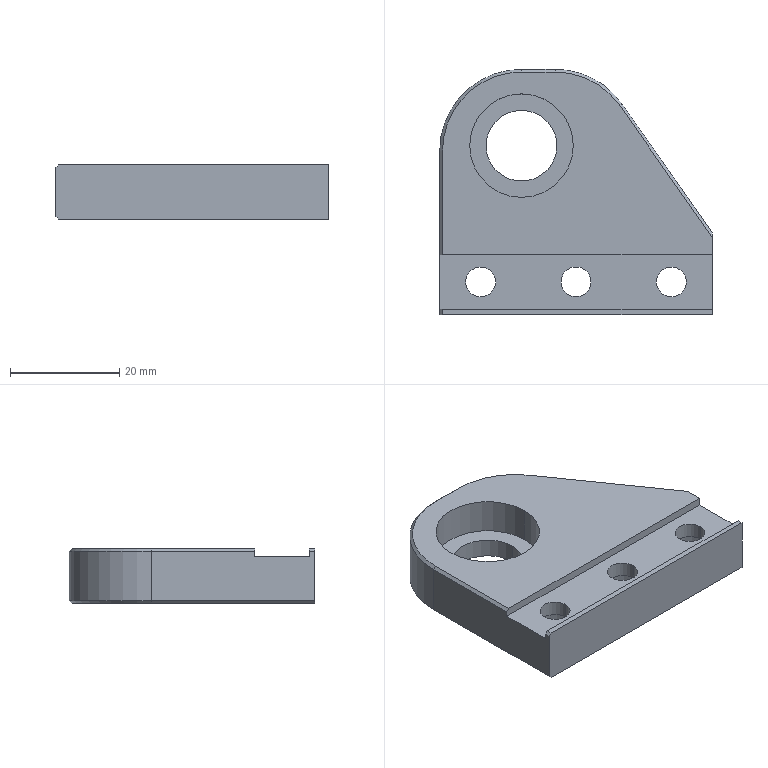Part | STEP file | 10000020492swp000-1 | 1 solid | 44 faces | box 50 x 45 x 10 mm | volume 14150 mm3 | plane 22 | cylinder 18 | cone 4 | commonest cylinder face diameters 5.5 x6 10 x6 13 x2 19 x2 30 x2
STEP:
#1=CARTESIAN_POINT('',(-19.5,8.5,3.5));
#2=VERTEX_POINT('',#1);
#3=CARTESIAN_POINT('',(-0.5,8.5,3.5));
#4=VERTEX_POINT('',#3);
#5=CARTESIAN_POINT('',(-10.,8.5,3.5));
#6=DIRECTION('',(0.,0.,1.));
#7=DIRECTION('',(1.,0.,0.));
#8=AXIS2_PLACEMENT_3D('',#5,#6,#7);
#9=CIRCLE('',#8,9.5);
#10=EDGE_CURVE('',#2,#4,#9,.T.);
#11=ORIENTED_EDGE('',*,*,#10,.F.);
#12=CARTESIAN_POINT('',(-19.5,8.5,10.));
#13=VERTEX_POINT('',#12);
#14=CARTESIAN_POINT('',(-19.5,8.5,10.));
#15=DIRECTION('',(0.,0.,1.));
#16=VECTOR('',#15,1000.);
#17=LINE('',#14,#16);
#18=EDGE_CURVE('',#2,#13,#17,.T.);
#19=ORIENTED_EDGE('',*,*,#18,.T.);
#20=CARTESIAN_POINT('',(-0.5,8.5,10.));
#21=VERTEX_POINT('',#20);
#22=CARTESIAN_POINT('',(-10.,8.5,10.));
#23=DIRECTION('',(0.,0.,1.));
#24=DIRECTION('',(1.,0.,0.));
#25=AXIS2_PLACEMENT_3D('',#22,#23,#24);
#26=CIRCLE('',#25,9.5);
#27=EDGE_CURVE('',#13,#21,#26,.T.);
#28=ORIENTED_EDGE('',*,*,#27,.T.);
#29=CARTESIAN_POINT('',(-0.5,8.5,10.));
#30=DIRECTION('',(0.,0.,1.));
#31=VECTOR('',#30,1000.);
#32=LINE('',#29,#31);
#33=EDGE_CURVE('',#4,#21,#32,.T.);
#34=ORIENTED_EDGE('',*,*,#33,.F.);
#35=EDGE_LOOP('',(#11,#19,#28,#34));
#36=FACE_OUTER_BOUND('',#35,.T.);
#37=CARTESIAN_POINT('',(-10.,8.5,10.));
#38=DIRECTION('',(0.,0.,1.));
#39=DIRECTION('',(1.,0.,0.));
#40=AXIS2_PLACEMENT_3D('',#37,#38,#39);
#41=CYLINDRICAL_SURFACE('',#40,9.5);
#42=ADVANCED_FACE('',(#36),#41,.F.);
#43=CARTESIAN_POINT('',(-16.5,8.5,0.));
#44=VERTEX_POINT('',#43);
#45=CARTESIAN_POINT('',(-3.5,8.5,0.));
#46=VERTEX_POINT('',#45);
#47=CARTESIAN_POINT('',(-10.,8.5,0.));
#48=DIRECTION('',(0.,0.,1.));
#49=DIRECTION('',(1.,0.,0.));
#50=AXIS2_PLACEMENT_3D('',#47,#48,#49);
#51=CIRCLE('',#50,6.5);
#52=EDGE_CURVE('',#44,#46,#51,.T.);
#53=ORIENTED_EDGE('',*,*,#52,.F.);
#54=CARTESIAN_POINT('',(-16.5,8.5,3.5));
#55=VERTEX_POINT('',#54);
#56=CARTESIAN_POINT('',(-16.5,8.5,10.));
#57=DIRECTION('',(0.,0.,1.));
#58=VECTOR('',#57,1000.);
#59=LINE('',#56,#58);
#60=EDGE_CURVE('',#44,#55,#59,.T.);
#61=ORIENTED_EDGE('',*,*,#60,.T.);
#62=CARTESIAN_POINT('',(-3.5,8.5,3.5));
#63=VERTEX_POINT('',#62);
#64=CARTESIAN_POINT('',(-10.,8.5,3.5));
#65=DIRECTION('',(0.,0.,1.));
#66=DIRECTION('',(1.,0.,0.));
#67=AXIS2_PLACEMENT_3D('',#64,#65,#66);
#68=CIRCLE('',#67,6.5);
#69=EDGE_CURVE('',#55,#63,#68,.T.);
#70=ORIENTED_EDGE('',*,*,#69,.T.);
#71=CARTESIAN_POINT('',(-3.5,8.5,10.));
#72=DIRECTION('',(0.,0.,1.));
#73=VECTOR('',#72,1000.);
#74=LINE('',#71,#73);
#75=EDGE_CURVE('',#46,#63,#74,.T.);
#76=ORIENTED_EDGE('',*,*,#75,.F.);
#77=EDGE_LOOP('',(#53,#61,#70,#76));
#78=FACE_OUTER_BOUND('',#77,.T.);
#79=CARTESIAN_POINT('',(-10.,8.5,10.));
#80=DIRECTION('',(0.,0.,1.));
#81=DIRECTION('',(1.,0.,0.));
#82=AXIS2_PLACEMENT_3D('',#79,#80,#81);
#83=CYLINDRICAL_SURFACE('',#82,6.5);
#84=ADVANCED_FACE('',(#78),#83,.F.);
#85=CARTESIAN_POINT('',(-12.5,-16.5,5.7));
#86=VERTEX_POINT('',#85);
#87=CARTESIAN_POINT('',(-22.5,-16.5,5.7));
#88=VERTEX_POINT('',#87);
#89=CARTESIAN_POINT('',(-17.5,-16.5,5.7));
#90=DIRECTION('',(0.,0.,-1.));
#91=DIRECTION('',(-1.,0.,0.));
#92=AXIS2_PLACEMENT_3D('',#89,#90,#91);
#93=CIRCLE('',#92,5.);
#94=EDGE_CURVE('',#86,#88,#93,.T.);
#95=ORIENTED_EDGE('',*,*,#94,.F.);
#96=CARTESIAN_POINT('',(-12.5,-16.5,0.));
#97=VERTEX_POINT('',#96);
#98=CARTESIAN_POINT('',(-12.5,-16.5,0.));
#99=DIRECTION('',(0.,0.,-1.));
#100=VECTOR('',#99,1000.);
#101=LINE('',#98,#100);
#102=EDGE_CURVE('',#86,#97,#101,.T.);
#103=ORIENTED_EDGE('',*,*,#102,.T.);
#104=CARTESIAN_POINT('',(-22.5,-16.5,0.));
#105=VERTEX_POINT('',#104);
#106=CARTESIAN_POINT('',(-17.5,-16.5,0.));
#107=DIRECTION('',(0.,0.,-1.));
#108=DIRECTION('',(-1.,0.,0.));
#109=AXIS2_PLACEMENT_3D('',#106,#107,#108);
#110=CIRCLE('',#109,5.);
#111=EDGE_CURVE('',#97,#105,#110,.T.);
#112=ORIENTED_EDGE('',*,*,#111,.T.);
#113=CARTESIAN_POINT('',(-22.5,-16.5,0.));
#114=DIRECTION('',(0.,0.,-1.));
#115=VECTOR('',#114,1000.);
#116=LINE('',#113,#115);
#117=EDGE_CURVE('',#88,#105,#116,.T.);
#118=ORIENTED_EDGE('',*,*,#117,.F.);
#119=EDGE_LOOP('',(#95,#103,#112,#118));
#120=FACE_OUTER_BOUND('',#119,.T.);
#121=CARTESIAN_POINT('',(-17.5,-16.5,0.));
#122=DIRECTION('',(0.,0.,-1.));
#123=DIRECTION('',(-1.,0.,0.));
#124=AXIS2_PLACEMENT_3D('',#121,#122,#123);
#125=CYLINDRICAL_SURFACE('',#124,5.);
#126=ADVANCED_FACE('',(#120),#125,.F.);
#127=CARTESIAN_POINT('',(-14.75,-16.5,8.5));
#128=VERTEX_POINT('',#127);
#129=CARTESIAN_POINT('',(-20.25,-16.5,8.5));
#130=VERTEX_POINT('',#129);
#131=CARTESIAN_POINT('',(-17.5,-16.5,8.5));
#132=DIRECTION('',(0.,0.,-1.));
#133=DIRECTION('',(-1.,0.,0.));
#134=AXIS2_PLACEMENT_3D('',#131,#132,#133);
#135=CIRCLE('',#134,2.75);
#136=EDGE_CURVE('',#128,#130,#135,.T.);
#137=ORIENTED_EDGE('',*,*,#136,.F.);
#138=CARTESIAN_POINT('',(-14.75,-16.5,5.7));
#139=VERTEX_POINT('',#138);
#140=CARTESIAN_POINT('',(-14.75,-16.5,0.));
#141=DIRECTION('',(0.,0.,-1.));
#142=VECTOR('',#141,1000.);
#143=LINE('',#140,#142);
#144=EDGE_CURVE('',#128,#139,#143,.T.);
#145=ORIENTED_EDGE('',*,*,#144,.T.);
#146=CARTESIAN_POINT('',(-20.25,-16.5,5.7));
#147=VERTEX_POINT('',#146);
#148=CARTESIAN_POINT('',(-17.5,-16.5,5.7));
#149=DIRECTION('',(0.,0.,-1.));
#150=DIRECTION('',(-1.,0.,0.));
#151=AXIS2_PLACEMENT_3D('',#148,#149,#150);
#152=CIRCLE('',#151,2.75);
#153=EDGE_CURVE('',#139,#147,#152,.T.);
#154=ORIENTED_EDGE('',*,*,#153,.T.);
#155=CARTESIAN_POINT('',(-20.25,-16.5,0.));
#156=DIRECTION('',(0.,0.,-1.));
#157=VECTOR('',#156,1000.);
#158=LINE('',#155,#157);
#159=EDGE_CURVE('',#130,#147,#158,.T.);
#160=ORIENTED_EDGE('',*,*,#159,.F.);
#161=EDGE_LOOP('',(#137,#145,#154,#160));
#162=FACE_OUTER_BOUND('',#161,.T.);
#163=CARTESIAN_POINT('',(-17.5,-16.5,0.));
#164=DIRECTION('',(0.,0.,-1.));
#165=DIRECTION('',(-1.,0.,0.));
#166=AXIS2_PLACEMENT_3D('',#163,#164,#165);
#167=CYLINDRICAL_SURFACE('',#166,2.75);
#168=ADVANCED_FACE('',(#162),#167,.F.);
#169=CARTESIAN_POINT('',(5.,-16.5,5.7));
#170=VERTEX_POINT('',#169);
#171=CARTESIAN_POINT('',(-5.,-16.5,5.7));
#172=VERTEX_POINT('',#171);
#173=CARTESIAN_POINT('',(0.,-16.5,5.7));
#174=DIRECTION('',(0.,0.,-1.));
#175=DIRECTION('',(-1.,0.,0.));
#176=AXIS2_PLACEMENT_3D('',#173,#174,#175);
#177=CIRCLE('',#176,5.);
#178=EDGE_CURVE('',#170,#172,#177,.T.);
#179=ORIENTED_EDGE('',*,*,#178,.F.);
#180=CARTESIAN_POINT('',(5.,-16.5,0.));
#181=VERTEX_POINT('',#180);
#182=CARTESIAN_POINT('',(5.,-16.5,0.));
#183=DIRECTION('',(0.,0.,-1.));
#184=VECTOR('',#183,1000.);
#185=LINE('',#182,#184);
#186=EDGE_CURVE('',#170,#181,#185,.T.);
#187=ORIENTED_EDGE('',*,*,#186,.T.);
#188=CARTESIAN_POINT('',(-5.,-16.5,0.));
#189=VERTEX_POINT('',#188);
#190=CARTESIAN_POINT('',(0.,-16.5,0.));
#191=DIRECTION('',(0.,0.,-1.));
#192=DIRECTION('',(-1.,0.,0.));
#193=AXIS2_PLACEMENT_3D('',#190,#191,#192);
#194=CIRCLE('',#193,5.);
#195=EDGE_CURVE('',#181,#189,#194,.T.);
#196=ORIENTED_EDGE('',*,*,#195,.T.);
#197=CARTESIAN_POINT('',(-5.,-16.5,0.));
#198=DIRECTION('',(0.,0.,-1.));
#199=VECTOR('',#198,1000.);
#200=LINE('',#197,#199);
#201=EDGE_CURVE('',#172,#189,#200,.T.);
#202=ORIENTED_EDGE('',*,*,#201,.F.);
#203=EDGE_LOOP('',(#179,#187,#196,#202));
#204=FACE_OUTER_BOUND('',#203,.T.);
#205=CARTESIAN_POINT('',(0.,-16.5,0.));
#206=DIRECTION('',(0.,0.,-1.));
#207=DIRECTION('',(-1.,0.,0.));
#208=AXIS2_PLACEMENT_3D('',#205,#206,#207);
#209=CYLINDRICAL_SURFACE('',#208,5.);
#210=ADVANCED_FACE('',(#204),#209,.F.);
#211=CARTESIAN_POINT('',(2.75,-16.5,8.5));
#212=VERTEX_POINT('',#211);
#213=CARTESIAN_POINT('',(-2.75,-16.5,8.5));
#214=VERTEX_POINT('',#213);
#215=CARTESIAN_POINT('',(0.,-16.5,8.5));
#216=DIRECTION('',(0.,0.,-1.));
#217=DIRECTION('',(-1.,0.,0.));
#218=AXIS2_PLACEMENT_3D('',#215,#216,#217);
#219=CIRCLE('',#218,2.75);
#220=EDGE_CURVE('',#212,#214,#219,.T.);
#221=ORIENTED_EDGE('',*,*,#220,.F.);
#222=CARTESIAN_POINT('',(2.75,-16.5,5.7));
#223=VERTEX_POINT('',#222);
#224=CARTESIAN_POINT('',(2.75,-16.5,0.));
#225=DIRECTION('',(0.,0.,-1.));
#226=VECTOR('',#225,1000.);
#227=LINE('',#224,#226);
#228=EDGE_CURVE('',#212,#223,#227,.T.);
#229=ORIENTED_EDGE('',*,*,#228,.T.);
#230=CARTESIAN_POINT('',(-2.75,-16.5,5.7));
#231=VERTEX_POINT('',#230);
#232=CARTESIAN_POINT('',(0.,-16.5,5.7));
#233=DIRECTION('',(0.,0.,-1.));
#234=DIRECTION('',(-1.,0.,0.));
#235=AXIS2_PLACEMENT_3D('',#232,#233,#234);
#236=CIRCLE('',#235,2.75);
#237=EDGE_CURVE('',#223,#231,#236,.T.);
#238=ORIENTED_EDGE('',*,*,#237,.T.);
#239=CARTESIAN_POINT('',(-2.75,-16.5,0.));
#240=DIRECTION('',(0.,0.,-1.));
#241=VECTOR('',#240,1000.);
#242=LINE('',#239,#241);
#243=EDGE_CURVE('',#214,#231,#242,.T.);
#244=ORIENTED_EDGE('',*,*,#243,.F.);
#245=EDGE_LOOP('',(#221,#229,#238,#244));
#246=FACE_OUTER_BOUND('',#245,.T.);
#247=CARTESIAN_POINT('',(0.,-16.5,0.));
#248=DIRECTION('',(0.,0.,-1.));
#249=DIRECTION('',(-1.,0.,0.));
#250=AXIS2_PLACEMENT_3D('',#247,#248,#249);
#251=CYLINDRICAL_SURFACE('',#250,2.75);
#252=ADVANCED_FACE('',(#246),#251,.F.);
#253=CARTESIAN_POINT('',(22.5,-16.5,5.7));
#254=VERTEX_POINT('',#253);
#255=CARTESIAN_POINT('',(12.5,-16.5,5.7));
#256=VERTEX_POINT('',#255);
#257=CARTESIAN_POINT('',(17.5,-16.5,5.7));
#258=DIRECTION('',(0.,0.,-1.));
#259=DIRECTION('',(-1.,0.,0.));
#260=AXIS2_PLACEMENT_3D('',#257,#258,#259);
#261=CIRCLE('',#260,5.);
#262=EDGE_CURVE('',#254,#256,#261,.T.);
#263=ORIENTED_EDGE('',*,*,#262,.F.);
#264=CARTESIAN_POINT('',(22.5,-16.5,0.));
#265=VERTEX_POINT('',#264);
#266=CARTESIAN_POINT('',(22.5,-16.5,0.));
#267=DIRECTION('',(0.,0.,-1.));
#268=VECTOR('',#267,1000.);
#269=LINE('',#266,#268);
#270=EDGE_CURVE('',#254,#265,#269,.T.);
#271=ORIENTED_EDGE('',*,*,#270,.T.);
#272=CARTESIAN_POINT('',(12.5,-16.5,0.));
#273=VERTEX_POINT('',#272);
#274=CARTESIAN_POINT('',(17.5,-16.5,0.));
#275=DIRECTION('',(0.,0.,-1.));
#276=DIRECTION('',(-1.,0.,0.));
#277=AXIS2_PLACEMENT_3D('',#274,#275,#276);
#278=CIRCLE('',#277,5.);
#279=EDGE_CURVE('',#265,#273,#278,.T.);
#280=ORIENTED_EDGE('',*,*,#279,.T.);
#281=CARTESIAN_POINT('',(12.5,-16.5,0.));
#282=DIRECTION('',(0.,0.,-1.));
#283=VECTOR('',#282,1000.);
#284=LINE('',#281,#283);
#285=EDGE_CURVE('',#256,#273,#284,.T.);
#286=ORIENTED_EDGE('',*,*,#285,.F.);
#287=EDGE_LOOP('',(#263,#271,#280,#286));
#288=FACE_OUTER_BOUND('',#287,.T.);
#289=CARTESIAN_POINT('',(17.5,-16.5,0.));
#290=DIRECTION('',(0.,0.,-1.));
#291=DIRECTION('',(-1.,0.,0.));
#292=AXIS2_PLACEMENT_3D('',#289,#290,#291);
#293=CYLINDRICAL_SURFACE('',#292,5.);
#294=ADVANCED_FACE('',(#288),#293,.F.);
#295=CARTESIAN_POINT('',(20.25,-16.5,8.5));
#296=VERTEX_POINT('',#295);
#297=CARTESIAN_POINT('',(14.75,-16.5,8.5));
#298=VERTEX_POINT('',#297);
#299=CARTESIAN_POINT('',(17.5,-16.5,8.5));
#300=DIRECTION('',(0.,0.,-1.));
#301=DIRECTION('',(-1.,0.,0.));
#302=AXIS2_PLACEMENT_3D('',#299,#300,#301);
#303=CIRCLE('',#302,2.75);
#304=EDGE_CURVE('',#296,#298,#303,.T.);
#305=ORIENTED_EDGE('',*,*,#304,.F.);
#306=CARTESIAN_POINT('',(20.25,-16.5,5.7));
#307=VERTEX_POINT('',#306);
#308=CARTESIAN_POINT('',(20.25,-16.5,0.));
#309=DIRECTION('',(0.,0.,-1.));
#310=VECTOR('',#309,1000.);
#311=LINE('',#308,#310);
#312=EDGE_CURVE('',#296,#307,#311,.T.);
#313=ORIENTED_EDGE('',*,*,#312,.T.);
#314=CARTESIAN_POINT('',(14.75,-16.5,5.7));
#315=VERTEX_POINT('',#314);
#316=CARTESIAN_POINT('',(17.5,-16.5,5.7));
#317=DIRECTION('',(0.,0.,-1.));
#318=DIRECTION('',(-1.,0.,0.));
#319=AXIS2_PLACEMENT_3D('',#316,#317,#318);
#320=CIRCLE('',#319,2.75);
#321=EDGE_CURVE('',#307,#315,#320,.T.);
#322=ORIENTED_EDGE('',*,*,#321,.T.);
#323=CARTESIAN_POINT('',(14.75,-16.5,0.));
#324=DIRECTION('',(0.,0.,-1.));
#325=VECTOR('',#324,1000.);
#326=LINE('',#323,#325);
#327=EDGE_CURVE('',#298,#315,#326,.T.);
#328=ORIENTED_EDGE('',*,*,#327,.F.);
#329=EDGE_LOOP('',(#305,#313,#322,#328));
#330=FACE_OUTER_BOUND('',#329,.T.);
#331=CARTESIAN_POINT('',(17.5,-16.5,0.));
#332=DIRECTION('',(0.,0.,-1.));
#333=DIRECTION('',(-1.,0.,0.));
#334=AXIS2_PLACEMENT_3D('',#331,#332,#333);
#335=CYLINDRICAL_SURFACE('',#334,2.75);
#336=ADVANCED_FACE('',(#330),#335,.F.);
#337=CARTESIAN_POINT('',(25.,-22.5,0.));
#338=VERTEX_POINT('',#337);
#339=CARTESIAN_POINT('',(25.,-8.372,0.));
#340=VERTEX_POINT('',#339);
#341=CARTESIAN_POINT('',(25.,22.5,0.));
#342=DIRECTION('',(0.,1.,0.));
#343=VECTOR('',#342,1000.);
#344=LINE('',#341,#343);
#345=EDGE_CURVE('',#338,#340,#344,.T.);
#346=ORIENTED_EDGE('',*,*,#345,.T.);
#347=CARTESIAN_POINT('',(25.,-7.5,0.5));
#348=VERTEX_POINT('',#347);
#349=CARTESIAN_POINT('',(25.,4.694,7.494));
#350=DIRECTION('',(0.,0.8674,0.4975));
#351=VECTOR('',#350,1000.);
#352=LINE('',#349,#351);
#353=EDGE_CURVE('',#340,#348,#352,.T.);
#354=ORIENTED_EDGE('',*,*,#353,.T.);
#355=CARTESIAN_POINT('',(25.,-7.5,9.5));
#356=VERTEX_POINT('',#355);
#357=CARTESIAN_POINT('',(25.,-7.5,0.));
#358=DIRECTION('',(0.,0.,1.));
#359=VECTOR('',#358,1000.);
#360=LINE('',#357,#359);
#361=EDGE_CURVE('',#348,#356,#360,.T.);
#362=ORIENTED_EDGE('',*,*,#361,.T.);
#363=CARTESIAN_POINT('',(25.,-8.372,10.));
#364=VERTEX_POINT('',#363);
#365=CARTESIAN_POINT('',(25.,15.074,-3.448));
#366=DIRECTION('',(0.,-0.8674,0.4975));
#367=VECTOR('',#366,1000.);
#368=LINE('',#365,#367);
#369=EDGE_CURVE('',#356,#364,#368,.T.);
#370=ORIENTED_EDGE('',*,*,#369,.T.);
#371=CARTESIAN_POINT('',(25.,-11.5,10.));
#372=VERTEX_POINT('',#371);
#373=CARTESIAN_POINT('',(25.,22.5,10.));
#374=DIRECTION('',(0.,1.,0.));
#375=VECTOR('',#374,1000.);
#376=LINE('',#373,#375);
#377=EDGE_CURVE('',#372,#364,#376,.T.);
#378=ORIENTED_EDGE('',*,*,#377,.F.);
#379=CARTESIAN_POINT('',(25.,-11.5,8.5));
#380=VERTEX_POINT('',#379);
#381=CARTESIAN_POINT('',(25.,-11.5,8.5));
#382=DIRECTION('',(0.,0.,1.));
#383=VECTOR('',#382,1000.);
#384=LINE('',#381,#383);
#385=EDGE_CURVE('',#380,#372,#384,.T.);
#386=ORIENTED_EDGE('',*,*,#385,.F.);
#387=CARTESIAN_POINT('',(25.,-21.5,8.5));
#388=VERTEX_POINT('',#387);
#389=CARTESIAN_POINT('',(25.,-11.5,8.5));
#390=DIRECTION('',(0.,-1.,0.));
#391=VECTOR('',#390,1000.);
#392=LINE('',#389,#391);
#393=EDGE_CURVE('',#380,#388,#392,.T.);
#394=ORIENTED_EDGE('',*,*,#393,.T.);
#395=CARTESIAN_POINT('',(25.,-21.5,10.));
#396=VERTEX_POINT('',#395);
#397=CARTESIAN_POINT('',(25.,-21.5,8.5));
#398=DIRECTION('',(0.,0.,1.));
#399=VECTOR('',#398,1000.);
#400=LINE('',#397,#399);
#401=EDGE_CURVE('',#388,#396,#400,.T.);
#402=ORIENTED_EDGE('',*,*,#401,.T.);
#403=CARTESIAN_POINT('',(25.,-22.5,10.));
#404=VERTEX_POINT('',#403);
#405=CARTESIAN_POINT('',(25.,22.5,10.));
#406=DIRECTION('',(0.,1.,0.));
#407=VECTOR('',#406,1000.);
#408=LINE('',#405,#407);
#409=EDGE_CURVE('',#404,#396,#408,.T.);
#410=ORIENTED_EDGE('',*,*,#409,.F.);
#411=CARTESIAN_POINT('',(25.,-22.5,10.));
#412=DIRECTION('',(0.,0.,-1.));
#413=VECTOR('',#412,1000.);
#414=LINE('',#411,#413);
#415=EDGE_CURVE('',#404,#338,#414,.T.);
#416=ORIENTED_EDGE('',*,*,#415,.T.);
#417=EDGE_LOOP('',(#346,#354,#362,#370,#378,#386,#394,#402,#410,#416));
#418=FACE_OUTER_BOUND('',#417,.T.);
#419=CARTESIAN_POINT('',(25.,22.5,10.));
#420=DIRECTION('',(-1.,0.,0.));
#421=DIRECTION('',(0.,-1.,0.));
#422=AXIS2_PLACEMENT_3D('',#419,#420,#421);
#423=PLANE('',#422);
#424=ADVANCED_FACE('',(#418),#423,.F.);
#425=CARTESIAN_POINT('',(-25.,-22.5,9.5));
#426=VERTEX_POINT('',#425);
#427=CARTESIAN_POINT('',(-25.,-22.5,0.5));
#428=VERTEX_POINT('',#427);
#429=CARTESIAN_POINT('',(-25.,-22.5,10.));
#430=DIRECTION('',(0.,0.,-1.));
#431=VECTOR('',#430,1000.);
#432=LINE('',#429,#431);
#433=EDGE_CURVE('',#426,#428,#432,.T.);
#434=ORIENTED_EDGE('',*,*,#433,.F.);
#435=CARTESIAN_POINT('',(-25.,-21.5,9.5));
#436=VERTEX_POINT('',#435);
#437=CARTESIAN_POINT('',(-25.,-21.5,9.5));
#438=DIRECTION('',(0.,1.,0.));
#439=VECTOR('',#438,1000.);
#440=LINE('',#437,#439);
#441=EDGE_CURVE('',#426,#436,#440,.T.);
#442=ORIENTED_EDGE('',*,*,#441,.T.);
#443=CARTESIAN_POINT('',(-25.,-21.5,8.5));
#444=VERTEX_POINT('',#443);
#445=CARTESIAN_POINT('',(-25.,-21.5,8.5));
#446=DIRECTION('',(0.,0.,1.));
#447=VECTOR('',#446,1000.);
#448=LINE('',#445,#447);
#449=EDGE_CURVE('',#444,#436,#448,.T.);
#450=ORIENTED_EDGE('',*,*,#449,.F.);
#451=CARTESIAN_POINT('',(-25.,-11.5,8.5));
#452=VERTEX_POINT('',#451);
#453=CARTESIAN_POINT('',(-25.,-11.5,8.5));
#454=DIRECTION('',(0.,1.,0.));
#455=VECTOR('',#454,1000.);
#456=LINE('',#453,#455);
#457=EDGE_CURVE('',#444,#452,#456,.T.);
#458=ORIENTED_EDGE('',*,*,#457,.T.);
#459=CARTESIAN_POINT('',(-25.,-11.5,9.5));
#460=VERTEX_POINT('',#459);
#461=CARTESIAN_POINT('',(-25.,-11.5,8.5));
#462=DIRECTION('',(0.,0.,1.));
#463=VECTOR('',#462,1000.);
#464=LINE('',#461,#463);
#465=EDGE_CURVE('',#452,#460,#464,.T.);
#466=ORIENTED_EDGE('',*,*,#465,.T.);
#467=CARTESIAN_POINT('',(-25.,7.5,9.5));
#468=VERTEX_POINT('',#467);
#469=CARTESIAN_POINT('',(-25.,7.5,9.5));
#470=DIRECTION('',(0.,1.,0.));
#471=VECTOR('',#470,1000.);
#472=LINE('',#469,#471);
#473=EDGE_CURVE('',#460,#468,#472,.T.);
#474=ORIENTED_EDGE('',*,*,#473,.T.);
#475=CARTESIAN_POINT('',(-25.,7.5,0.5));
#476=VERTEX_POINT('',#475);
#477=CARTESIAN_POINT('',(-25.,7.5,10.));
#478=DIRECTION('',(0.,0.,-1.));
#479=VECTOR('',#478,1000.);
#480=LINE('',#477,#479);
#481=EDGE_CURVE('',#468,#476,#480,.T.);
#482=ORIENTED_EDGE('',*,*,#481,.T.);
#483=CARTESIAN_POINT('',(-25.,22.5,0.5));
#484=DIRECTION('',(0.,-1.,0.));
#485=VECTOR('',#484,1000.);
#486=LINE('',#483,#485);
#487=EDGE_CURVE('',#476,#428,#486,.T.);
#488=ORIENTED_EDGE('',*,*,#487,.T.);
#489=EDGE_LOOP('',(#434,#442,#450,#458,#466,#474,#482,#488));
#490=FACE_OUTER_BOUND('',#489,.T.);
#491=CARTESIAN_POINT('',(-25.,22.5,10.));
#492=DIRECTION('',(1.,0.,0.));
#493=DIRECTION('',(0.,1.,0.));
#494=AXIS2_PLACEMENT_3D('',#491,#492,#493);
#495=PLANE('',#494);
#496=ADVANCED_FACE('',(#490),#495,.F.);
#497=CARTESIAN_POINT('',(-24.5,-21.5,10.));
#498=VERTEX_POINT('',#497);
#499=CARTESIAN_POINT('',(25.,-21.5,10.));
#500=DIRECTION('',(-1.,0.,0.));
#501=VECTOR('',#500,1000.);
#502=LINE('',#499,#501);
#503=EDGE_CURVE('',#396,#498,#502,.T.);
#504=ORIENTED_EDGE('',*,*,#503,.T.);
#505=CARTESIAN_POINT('',(-24.5,-22.5,10.));
#506=VERTEX_POINT('',#505);
#507=CARTESIAN_POINT('',(-24.5,-22.5,10.));
#508=DIRECTION('',(0.,-1.,0.));
#509=VECTOR('',#508,1000.);
#510=LINE('',#507,#509);
#511=EDGE_CURVE('',#498,#506,#510,.T.);
#512=ORIENTED_EDGE('',*,*,#511,.T.);
#513=CARTESIAN_POINT('',(-25.,-22.5,10.));
#514=DIRECTION('',(1.,0.,0.));
#515=VECTOR('',#514,1000.);
#516=LINE('',#513,#515);
#517=EDGE_CURVE('',#506,#404,#516,.T.);
#518=ORIENTED_EDGE('',*,*,#517,.T.);
#519=ORIENTED_EDGE('',*,*,#409,.T.);
#520=EDGE_LOOP('',(#504,#512,#518,#519));
#521=FACE_OUTER_BOUND('',#520,.T.);
#522=CARTESIAN_POINT('',(0.,0.,10.));
#523=DIRECTION('',(0.,0.,1.));
#524=DIRECTION('',(1.,0.,0.));
#525=AXIS2_PLACEMENT_3D('',#522,#523,#524);
#526=PLANE('',#525);
#527=ADVANCED_FACE('',(#521),#526,.T.);
#528=ORIENTED_EDGE('',*,*,#377,.T.);
#529=CARTESIAN_POINT('',(8.063,15.817,10.));
#530=VERTEX_POINT('',#529);
#531=CARTESIAN_POINT('',(8.063,15.817,10.));
#532=DIRECTION('',(-0.5736,0.8192,0.));
#533=VECTOR('',#532,1000.);
#534=LINE('',#531,#533);
#535=EDGE_CURVE('',#364,#530,#534,.T.);
#536=ORIENTED_EDGE('',*,*,#535,.T.);
#537=CARTESIAN_POINT('',(-3.815,22.,10.));
#538=VERTEX_POINT('',#537);
#539=CARTESIAN_POINT('',(-3.815,7.5,10.));
#540=DIRECTION('',(0.,0.,1.));
#541=DIRECTION('',(1.,0.,0.));
#542=AXIS2_PLACEMENT_3D('',#539,#540,#541);
#543=CIRCLE('',#542,14.5);
#544=EDGE_CURVE('',#530,#538,#543,.T.);
#545=ORIENTED_EDGE('',*,*,#544,.T.);
#546=CARTESIAN_POINT('',(-10.,22.,10.));
#547=VERTEX_POINT('',#546);
#548=CARTESIAN_POINT('',(-10.,22.,10.));
#549=DIRECTION('',(-1.,0.,0.));
#550=VECTOR('',#549,1000.);
#551=LINE('',#548,#550);
#552=EDGE_CURVE('',#538,#547,#551,.T.);
#553=ORIENTED_EDGE('',*,*,#552,.T.);
#554=CARTESIAN_POINT('',(-24.5,7.5,10.));
#555=VERTEX_POINT('',#554);
#556=CARTESIAN_POINT('',(-10.,7.5,10.));
#557=DIRECTION('',(0.,0.,1.));
#558=DIRECTION('',(1.,0.,0.));
#559=AXIS2_PLACEMENT_3D('',#556,#557,#558);
#560=CIRCLE('',#559,14.5);
#561=EDGE_CURVE('',#547,#555,#560,.T.);
#562=ORIENTED_EDGE('',*,*,#561,.T.);
#563=CARTESIAN_POINT('',(-24.5,-11.5,10.));
#564=VERTEX_POINT('',#563);
#565=CARTESIAN_POINT('',(-24.5,-11.5,10.));
#566=DIRECTION('',(0.,-1.,0.));
#567=VECTOR('',#566,1000.);
#568=LINE('',#565,#567);
#569=EDGE_CURVE('',#555,#564,#568,.T.);
#570=ORIENTED_EDGE('',*,*,#569,.T.);
#571=CARTESIAN_POINT('',(25.,-11.5,10.));
#572=DIRECTION('',(1.,0.,0.));
#573=VECTOR('',#572,1000.);
#574=LINE('',#571,#573);
#575=EDGE_CURVE('',#564,#372,#574,.T.);
#576=ORIENTED_EDGE('',*,*,#575,.T.);
#577=EDGE_LOOP('',(#528,#536,#545,#553,#562,#570,#576));
#578=FACE_OUTER_BOUND('',#577,.T.);
#579=CARTESIAN_POINT('',(-10.,8.5,10.));
#580=DIRECTION('',(0.,0.,1.));
#581=DIRECTION('',(1.,0.,0.));
#582=AXIS2_PLACEMENT_3D('',#579,#580,#581);
#583=CIRCLE('',#582,9.5);
#584=EDGE_CURVE('',#21,#13,#583,.T.);
#585=ORIENTED_EDGE('',*,*,#584,.F.);
#586=ORIENTED_EDGE('',*,*,#27,.F.);
#587=EDGE_LOOP('',(#585,#586));
#588=FACE_BOUND('',#587,.T.);
#589=CARTESIAN_POINT('',(0.,0.,10.));
#590=DIRECTION('',(0.,0.,1.));
#591=DIRECTION('',(1.,0.,0.));
#592=AXIS2_PLACEMENT_3D('',#589,#590,#591);
#593=PLANE('',#592);
#594=ADVANCED_FACE('',(#578,#588),#593,.T.);
#595=CARTESIAN_POINT('',(-3.815,22.5,9.5));
#596=VERTEX_POINT('',#595);
#597=CARTESIAN_POINT('',(-3.815,22.5,0.5));
#598=VERTEX_POINT('',#597);
#599=CARTESIAN_POINT('',(-3.815,22.5,10.));
#600=DIRECTION('',(0.,0.,-1.));
#601=VECTOR('',#600,1000.);
#602=LINE('',#599,#601);
#603=EDGE_CURVE('',#596,#598,#602,.T.);
#604=ORIENTED_EDGE('',*,*,#603,.T.);
#605=CARTESIAN_POINT('',(-10.,22.5,0.5));
#606=VERTEX_POINT('',#605);
#607=CARTESIAN_POINT('',(-25.,22.5,0.5));
#608=DIRECTION('',(-1.,0.,0.));
#609=VECTOR('',#608,1000.);
#610=LINE('',#607,#609);
#611=EDGE_CURVE('',#598,#606,#610,.T.);
#612=ORIENTED_EDGE('',*,*,#611,.T.);
#613=CARTESIAN_POINT('',(-10.,22.5,9.5));
#614=VERTEX_POINT('',#613);
#615=CARTESIAN_POINT('',(-10.,22.5,10.));
#616=DIRECTION('',(0.,0.,1.));
#617=VECTOR('',#616,1000.);
#618=LINE('',#615,#617);
#619=EDGE_CURVE('',#606,#614,#618,.T.);
#620=ORIENTED_EDGE('',*,*,#619,.T.);
#621=CARTESIAN_POINT('',(-3.815,22.5,9.5));
#622=DIRECTION('',(1.,0.,0.));
#623=VECTOR('',#622,1000.);
#624=LINE('',#621,#623);
#625=EDGE_CURVE('',#614,#596,#624,.T.);
#626=ORIENTED_EDGE('',*,*,#625,.T.);
#627=EDGE_LOOP('',(#604,#612,#620,#626));
#628=FACE_OUTER_BOUND('',#627,.T.);
#629=CARTESIAN_POINT('',(-25.,22.5,10.));
#630=DIRECTION('',(0.,-1.,0.));
#631=DIRECTION('',(0.,0.,-1.));
#632=AXIS2_PLACEMENT_3D('',#629,#630,#631);
#633=PLANE('',#632);
#634=ADVANCED_FACE('',(#628),#633,.F.);
#635=ORIENTED_EDGE('',*,*,#517,.F.);
#636=CARTESIAN_POINT('',(-24.5,-22.5,10.));
#637=DIRECTION('',(-0.7071,0.,-0.7071));
#638=VECTOR('',#637,1000.);
#639=LINE('',#636,#638);
#640=EDGE_CURVE('',#506,#426,#639,.T.);
#641=ORIENTED_EDGE('',*,*,#640,.T.);
#642=ORIENTED_EDGE('',*,*,#433,.T.);
#643=CARTESIAN_POINT('',(-24.5,-22.5,0.));
#644=VERTEX_POINT('',#643);
#645=CARTESIAN_POINT('',(-25.,-22.5,0.5));
#646=DIRECTION('',(0.7071,0.,-0.7071));
#647=VECTOR('',#646,1000.);
#648=LINE('',#645,#647);
#649=EDGE_CURVE('',#428,#644,#648,.T.);
#650=ORIENTED_EDGE('',*,*,#649,.T.);
#651=CARTESIAN_POINT('',(-25.,-22.5,0.));
#652=DIRECTION('',(1.,0.,0.));
#653=VECTOR('',#652,1000.);
#654=LINE('',#651,#653);
#655=EDGE_CURVE('',#644,#338,#654,.T.);
#656=ORIENTED_EDGE('',*,*,#655,.T.);
#657=ORIENTED_EDGE('',*,*,#415,.F.);
#658=EDGE_LOOP('',(#635,#641,#642,#650,#656,#657));
#659=FACE_OUTER_BOUND('',#658,.T.);
#660=CARTESIAN_POINT('',(-25.,-22.5,10.));
#661=DIRECTION('',(0.,1.,0.));
#662=DIRECTION('',(0.,0.,1.));
#663=AXIS2_PLACEMENT_3D('',#660,#661,#662);
#664=PLANE('',#663);
#665=ADVANCED_FACE('',(#659),#664,.F.);
#666=CARTESIAN_POINT('',(-10.,8.5,0.));
#667=DIRECTION('',(0.,0.,1.));
#668=DIRECTION('',(1.,0.,0.));
#669=AXIS2_PLACEMENT_3D('',#666,#667,#668);
#670=CIRCLE('',#669,6.5);
#671=EDGE_CURVE('',#46,#44,#670,.T.);
#672=ORIENTED_EDGE('',*,*,#671,.T.);
#673=ORIENTED_EDGE('',*,*,#52,.T.);
#674=EDGE_LOOP('',(#672,#673));
#675=FACE_BOUND('',#674,.T.);
#676=CARTESIAN_POINT('',(-17.5,-16.5,0.));
#677=DIRECTION('',(0.,0.,-1.));
#678=DIRECTION('',(-1.,0.,0.));
#679=AXIS2_PLACEMENT_3D('',#676,#677,#678);
#680=CIRCLE('',#679,5.);
#681=EDGE_CURVE('',#105,#97,#680,.T.);
#682=ORIENTED_EDGE('',*,*,#681,.F.);
#683=ORIENTED_EDGE('',*,*,#111,.F.);
#684=EDGE_LOOP('',(#682,#683));
#685=FACE_BOUND('',#684,.T.);
#686=CARTESIAN_POINT('',(0.,-16.5,0.));
#687=DIRECTION('',(0.,0.,-1.));
#688=DIRECTION('',(-1.,0.,0.));
#689=AXIS2_PLACEMENT_3D('',#686,#687,#688);
#690=CIRCLE('',#689,5.);
#691=EDGE_CURVE('',#189,#181,#690,.T.);
#692=ORIENTED_EDGE('',*,*,#691,.F.);
#693=ORIENTED_EDGE('',*,*,#195,.F.);
#694=EDGE_LOOP('',(#692,#693));
#695=FACE_BOUND('',#694,.T.);
#696=CARTESIAN_POINT('',(17.5,-16.5,0.));
#697=DIRECTION('',(0.,0.,-1.));
#698=DIRECTION('',(-1.,0.,0.));
#699=AXIS2_PLACEMENT_3D('',#696,#697,#698);
#700=CIRCLE('',#699,5.);
#701=EDGE_CURVE('',#273,#265,#700,.T.);
#702=ORIENTED_EDGE('',*,*,#701,.F.);
#703=ORIENTED_EDGE('',*,*,#279,.F.);
#704=EDGE_LOOP('',(#702,#703));
#705=FACE_BOUND('',#704,.T.);
#706=CARTESIAN_POINT('',(-3.815,22.,0.));
#707=VERTEX_POINT('',#706);
#708=CARTESIAN_POINT('',(8.063,15.817,0.));
#709=VERTEX_POINT('',#708);
#710=CARTESIAN_POINT('',(-3.815,7.5,0.));
#711=DIRECTION('',(0.,0.,-1.));
#712=DIRECTION('',(1.,0.,0.));
#713=AXIS2_PLACEMENT_3D('',#710,#711,#712);
#714=CIRCLE('',#713,14.5);
#715=EDGE_CURVE('',#707,#709,#714,.T.);
#716=ORIENTED_EDGE('',*,*,#715,.T.);
#717=CARTESIAN_POINT('',(12.842,8.992,0.));
#718=DIRECTION('',(0.5736,-0.8192,0.));
#719=VECTOR('',#718,1000.);
#720=LINE('',#717,#719);
#721=EDGE_CURVE('',#709,#340,#720,.T.);
#722=ORIENTED_EDGE('',*,*,#721,.T.);
#723=ORIENTED_EDGE('',*,*,#345,.F.);
#724=ORIENTED_EDGE('',*,*,#655,.F.);
#725=CARTESIAN_POINT('',(-24.5,7.5,0.));
#726=VERTEX_POINT('',#725);
#727=CARTESIAN_POINT('',(-24.5,0.,0.));
#728=DIRECTION('',(0.,1.,0.));
#729=VECTOR('',#728,1000.);
#730=LINE('',#727,#729);
#731=EDGE_CURVE('',#644,#726,#730,.T.);
#732=ORIENTED_EDGE('',*,*,#731,.T.);
#733=CARTESIAN_POINT('',(-10.,22.,0.));
#734=VERTEX_POINT('',#733);
#735=CARTESIAN_POINT('',(-10.,7.5,0.));
#736=DIRECTION('',(0.,0.,-1.));
#737=DIRECTION('',(1.,0.,0.));
#738=AXIS2_PLACEMENT_3D('',#735,#736,#737);
#739=CIRCLE('',#738,14.5);
#740=EDGE_CURVE('',#726,#734,#739,.T.);
#741=ORIENTED_EDGE('',*,*,#740,.T.);
#742=CARTESIAN_POINT('',(0.,22.,0.));
#743=DIRECTION('',(1.,0.,0.));
#744=VECTOR('',#743,1000.);
#745=LINE('',#742,#744);
#746=EDGE_CURVE('',#734,#707,#745,.T.);
#747=ORIENTED_EDGE('',*,*,#746,.T.);
#748=EDGE_LOOP('',(#716,#722,#723,#724,#732,#741,#747));
#749=FACE_OUTER_BOUND('',#748,.T.);
#750=CARTESIAN_POINT('',(0.,0.,0.));
#751=DIRECTION('',(0.,0.,1.));
#752=DIRECTION('',(1.,0.,0.));
#753=AXIS2_PLACEMENT_3D('',#750,#751,#752);
#754=PLANE('',#753);
#755=ADVANCED_FACE('',(#675,#685,#695,#705,#749),#754,.F.);
#756=ORIENTED_EDGE('',*,*,#361,.F.);
#757=CARTESIAN_POINT('',(8.473,16.104,0.5));
#758=VERTEX_POINT('',#757);
#759=CARTESIAN_POINT('',(3.994,22.5,0.5));
#760=DIRECTION('',(-0.5736,0.8192,0.));
#761=VECTOR('',#760,1000.);
#762=LINE('',#759,#761);
#763=EDGE_CURVE('',#348,#758,#762,.T.);
#764=ORIENTED_EDGE('',*,*,#763,.T.);
#765=CARTESIAN_POINT('',(8.473,16.104,9.5));
#766=VERTEX_POINT('',#765);
#767=CARTESIAN_POINT('',(8.473,16.104,0.));
#768=DIRECTION('',(0.,0.,1.));
#769=VECTOR('',#768,1000.);
#770=LINE('',#767,#769);
#771=EDGE_CURVE('',#758,#766,#770,.T.);
#772=ORIENTED_EDGE('',*,*,#771,.T.);
#773=CARTESIAN_POINT('',(25.,-7.5,9.5));
#774=DIRECTION('',(0.5736,-0.8192,0.));
#775=VECTOR('',#774,1000.);
#776=LINE('',#773,#775);
#777=EDGE_CURVE('',#766,#356,#776,.T.);
#778=ORIENTED_EDGE('',*,*,#777,.T.);
#779=EDGE_LOOP('',(#756,#764,#772,#778));
#780=FACE_OUTER_BOUND('',#779,.T.);
#781=CARTESIAN_POINT('',(3.994,22.5,0.));
#782=DIRECTION('',(-0.8192,-0.5736,0.));
#783=DIRECTION('',(0.5736,-0.8192,0.));
#784=AXIS2_PLACEMENT_3D('',#781,#782,#783);
#785=PLANE('',#784);
#786=ADVANCED_FACE('',(#780),#785,.F.);
#787=ORIENTED_EDGE('',*,*,#449,.T.);
#788=CARTESIAN_POINT('',(-0.5,-21.5,34.));
#789=DIRECTION('',(0.7071,0.,0.7071));
#790=VECTOR('',#789,1000.);
#791=LINE('',#788,#790);
#792=EDGE_CURVE('',#436,#498,#791,.T.);
#793=ORIENTED_EDGE('',*,*,#792,.T.);
#794=ORIENTED_EDGE('',*,*,#503,.F.);
#795=ORIENTED_EDGE('',*,*,#401,.F.);
#796=CARTESIAN_POINT('',(25.,-21.5,8.5));
#797=DIRECTION('',(-1.,0.,0.));
#798=VECTOR('',#797,1000.);
#799=LINE('',#796,#798);
#800=EDGE_CURVE('',#388,#444,#799,.T.);
#801=ORIENTED_EDGE('',*,*,#800,.T.);
#802=EDGE_LOOP('',(#787,#793,#794,#795,#801));
#803=FACE_OUTER_BOUND('',#802,.T.);
#804=CARTESIAN_POINT('',(25.,-21.5,8.5));
#805=DIRECTION('',(0.,1.,0.));
#806=DIRECTION('',(0.,0.,1.));
#807=AXIS2_PLACEMENT_3D('',#804,#805,#806);
#808=PLANE('',#807);
#809=ADVANCED_FACE('',(#803),#808,.T.);
#810=ORIENTED_EDGE('',*,*,#575,.F.);
#811=CARTESIAN_POINT('',(-0.5,-11.5,34.));
#812=DIRECTION('',(-0.7071,0.,-0.7071));
#813=VECTOR('',#812,1000.);
#814=LINE('',#811,#813);
#815=EDGE_CURVE('',#564,#460,#814,.T.);
#816=ORIENTED_EDGE('',*,*,#815,.T.);
#817=ORIENTED_EDGE('',*,*,#465,.F.);
#818=CARTESIAN_POINT('',(25.,-11.5,8.5));
#819=DIRECTION('',(1.,0.,0.));
#820=VECTOR('',#819,1000.);
#821=LINE('',#818,#820);
#822=EDGE_CURVE('',#452,#380,#821,.T.);
#823=ORIENTED_EDGE('',*,*,#822,.T.);
#824=ORIENTED_EDGE('',*,*,#385,.T.);
#825=EDGE_LOOP('',(#810,#816,#817,#823,#824));
#826=FACE_OUTER_BOUND('',#825,.T.);
#827=CARTESIAN_POINT('',(25.,-11.5,8.5));
#828=DIRECTION('',(0.,-1.,0.));
#829=DIRECTION('',(0.,0.,-1.));
#830=AXIS2_PLACEMENT_3D('',#827,#828,#829);
#831=PLANE('',#830);
#832=ADVANCED_FACE('',(#826),#831,.T.);
#833=CARTESIAN_POINT('',(-17.5,-16.5,8.5));
#834=DIRECTION('',(0.,0.,-1.));
#835=DIRECTION('',(-1.,0.,0.));
#836=AXIS2_PLACEMENT_3D('',#833,#834,#835);
#837=CIRCLE('',#836,2.75);
#838=EDGE_CURVE('',#130,#128,#837,.T.);
#839=ORIENTED_EDGE('',*,*,#838,.T.);
#840=ORIENTED_EDGE('',*,*,#136,.T.);
#841=EDGE_LOOP('',(#839,#840));
#842=FACE_BOUND('',#841,.T.);
#843=CARTESIAN_POINT('',(0.,-16.5,8.5));
#844=DIRECTION('',(0.,0.,-1.));
#845=DIRECTION('',(-1.,0.,0.));
#846=AXIS2_PLACEMENT_3D('',#843,#844,#845);
#847=CIRCLE('',#846,2.75);
#848=EDGE_CURVE('',#214,#212,#847,.T.);
#849=ORIENTED_EDGE('',*,*,#848,.T.);
#850=ORIENTED_EDGE('',*,*,#220,.T.);
#851=EDGE_LOOP('',(#849,#850));
#852=FACE_BOUND('',#851,.T.);
#853=CARTESIAN_POINT('',(17.5,-16.5,8.5));
#854=DIRECTION('',(0.,0.,-1.));
#855=DIRECTION('',(-1.,0.,0.));
#856=AXIS2_PLACEMENT_3D('',#853,#854,#855);
#857=CIRCLE('',#856,2.75);
#858=EDGE_CURVE('',#298,#296,#857,.T.);
#859=ORIENTED_EDGE('',*,*,#858,.T.);
#860=ORIENTED_EDGE('',*,*,#304,.T.);
#861=EDGE_LOOP('',(#859,#860));
#862=FACE_BOUND('',#861,.T.);
#863=ORIENTED_EDGE('',*,*,#393,.F.);
#864=ORIENTED_EDGE('',*,*,#822,.F.);
#865=ORIENTED_EDGE('',*,*,#457,.F.);
#866=ORIENTED_EDGE('',*,*,#800,.F.);
#867=EDGE_LOOP('',(#863,#864,#865,#866));
#868=FACE_OUTER_BOUND('',#867,.T.);
#869=CARTESIAN_POINT('',(0.,0.,8.5));
#870=DIRECTION('',(0.,0.,-1.));
#871=DIRECTION('',(-1.,0.,0.));
#872=AXIS2_PLACEMENT_3D('',#869,#870,#871);
#873=PLANE('',#872);
#874=ADVANCED_FACE('',(#842,#852,#862,#868),#873,.F.);
#875=ORIENTED_EDGE('',*,*,#312,.F.);
#876=ORIENTED_EDGE('',*,*,#858,.F.);
#877=ORIENTED_EDGE('',*,*,#327,.T.);
#878=CARTESIAN_POINT('',(17.5,-16.5,5.7));
#879=DIRECTION('',(0.,0.,-1.));
#880=DIRECTION('',(-1.,0.,0.));
#881=AXIS2_PLACEMENT_3D('',#878,#879,#880);
#882=CIRCLE('',#881,2.75);
#883=EDGE_CURVE('',#315,#307,#882,.T.);
#884=ORIENTED_EDGE('',*,*,#883,.T.);
#885=EDGE_LOOP('',(#875,#876,#877,#884));
#886=FACE_OUTER_BOUND('',#885,.T.);
#887=CARTESIAN_POINT('',(17.5,-16.5,0.));
#888=DIRECTION('',(0.,0.,-1.));
#889=DIRECTION('',(-1.,0.,0.));
#890=AXIS2_PLACEMENT_3D('',#887,#888,#889);
#891=CYLINDRICAL_SURFACE('',#890,2.75);
#892=ADVANCED_FACE('',(#886),#891,.F.);
#893=ORIENTED_EDGE('',*,*,#883,.F.);
#894=ORIENTED_EDGE('',*,*,#321,.F.);
#895=EDGE_LOOP('',(#893,#894));
#896=FACE_BOUND('',#895,.T.);
#897=CARTESIAN_POINT('',(17.5,-16.5,5.7));
#898=DIRECTION('',(0.,0.,-1.));
#899=DIRECTION('',(-1.,0.,0.));
#900=AXIS2_PLACEMENT_3D('',#897,#898,#899);
#901=CIRCLE('',#900,5.);
#902=EDGE_CURVE('',#256,#254,#901,.T.);
#903=ORIENTED_EDGE('',*,*,#902,.T.);
#904=ORIENTED_EDGE('',*,*,#262,.T.);
#905=EDGE_LOOP('',(#903,#904));
#906=FACE_OUTER_BOUND('',#905,.T.);
#907=CARTESIAN_POINT('',(20.25,-16.5,5.7));
#908=DIRECTION('',(0.,0.,1.));
#909=DIRECTION('',(1.,0.,0.));
#910=AXIS2_PLACEMENT_3D('',#907,#908,#909);
#911=PLANE('',#910);
#912=ADVANCED_FACE('',(#896,#906),#911,.F.);
#913=ORIENTED_EDGE('',*,*,#270,.F.);
#914=ORIENTED_EDGE('',*,*,#902,.F.);
#915=ORIENTED_EDGE('',*,*,#285,.T.);
#916=ORIENTED_EDGE('',*,*,#701,.T.);
#917=EDGE_LOOP('',(#913,#914,#915,#916));
#918=FACE_OUTER_BOUND('',#917,.T.);
#919=CARTESIAN_POINT('',(17.5,-16.5,0.));
#920=DIRECTION('',(0.,0.,-1.));
#921=DIRECTION('',(-1.,0.,0.));
#922=AXIS2_PLACEMENT_3D('',#919,#920,#921);
#923=CYLINDRICAL_SURFACE('',#922,5.);
#924=ADVANCED_FACE('',(#918),#923,.F.);
#925=ORIENTED_EDGE('',*,*,#228,.F.);
#926=ORIENTED_EDGE('',*,*,#848,.F.);
#927=ORIENTED_EDGE('',*,*,#243,.T.);
#928=CARTESIAN_POINT('',(0.,-16.5,5.7));
#929=DIRECTION('',(0.,0.,-1.));
#930=DIRECTION('',(-1.,0.,0.));
#931=AXIS2_PLACEMENT_3D('',#928,#929,#930);
#932=CIRCLE('',#931,2.75);
#933=EDGE_CURVE('',#231,#223,#932,.T.);
#934=ORIENTED_EDGE('',*,*,#933,.T.);
#935=EDGE_LOOP('',(#925,#926,#927,#934));
#936=FACE_OUTER_BOUND('',#935,.T.);
#937=CARTESIAN_POINT('',(0.,-16.5,0.));
#938=DIRECTION('',(0.,0.,-1.));
#939=DIRECTION('',(-1.,0.,0.));
#940=AXIS2_PLACEMENT_3D('',#937,#938,#939);
#941=CYLINDRICAL_SURFACE('',#940,2.75);
#942=ADVANCED_FACE('',(#936),#941,.F.);
#943=ORIENTED_EDGE('',*,*,#933,.F.);
#944=ORIENTED_EDGE('',*,*,#237,.F.);
#945=EDGE_LOOP('',(#943,#944));
#946=FACE_BOUND('',#945,.T.);
#947=CARTESIAN_POINT('',(0.,-16.5,5.7));
#948=DIRECTION('',(0.,0.,-1.));
#949=DIRECTION('',(-1.,0.,0.));
#950=AXIS2_PLACEMENT_3D('',#947,#948,#949);
#951=CIRCLE('',#950,5.);
#952=EDGE_CURVE('',#172,#170,#951,.T.);
#953=ORIENTED_EDGE('',*,*,#952,.T.);
#954=ORIENTED_EDGE('',*,*,#178,.T.);
#955=EDGE_LOOP('',(#953,#954));
#956=FACE_OUTER_BOUND('',#955,.T.);
#957=CARTESIAN_POINT('',(2.75,-16.5,5.7));
#958=DIRECTION('',(0.,0.,1.));
#959=DIRECTION('',(1.,0.,0.));
#960=AXIS2_PLACEMENT_3D('',#957,#958,#959);
#961=PLANE('',#960);
#962=ADVANCED_FACE('',(#946,#956),#961,.F.);
#963=ORIENTED_EDGE('',*,*,#186,.F.);
#964=ORIENTED_EDGE('',*,*,#952,.F.);
#965=ORIENTED_EDGE('',*,*,#201,.T.);
#966=ORIENTED_EDGE('',*,*,#691,.T.);
#967=EDGE_LOOP('',(#963,#964,#965,#966));
#968=FACE_OUTER_BOUND('',#967,.T.);
#969=CARTESIAN_POINT('',(0.,-16.5,0.));
#970=DIRECTION('',(0.,0.,-1.));
#971=DIRECTION('',(-1.,0.,0.));
#972=AXIS2_PLACEMENT_3D('',#969,#970,#971);
#973=CYLINDRICAL_SURFACE('',#972,5.);
#974=ADVANCED_FACE('',(#968),#973,.F.);
#975=ORIENTED_EDGE('',*,*,#144,.F.);
#976=ORIENTED_EDGE('',*,*,#838,.F.);
#977=ORIENTED_EDGE('',*,*,#159,.T.);
#978=CARTESIAN_POINT('',(-17.5,-16.5,5.7));
#979=DIRECTION('',(0.,0.,-1.));
#980=DIRECTION('',(-1.,0.,0.));
#981=AXIS2_PLACEMENT_3D('',#978,#979,#980);
#982=CIRCLE('',#981,2.75);
#983=EDGE_CURVE('',#147,#139,#982,.T.);
#984=ORIENTED_EDGE('',*,*,#983,.T.);
#985=EDGE_LOOP('',(#975,#976,#977,#984));
#986=FACE_OUTER_BOUND('',#985,.T.);
#987=CARTESIAN_POINT('',(-17.5,-16.5,0.));
#988=DIRECTION('',(0.,0.,-1.));
#989=DIRECTION('',(-1.,0.,0.));
#990=AXIS2_PLACEMENT_3D('',#987,#988,#989);
#991=CYLINDRICAL_SURFACE('',#990,2.75);
#992=ADVANCED_FACE('',(#986),#991,.F.);
#993=ORIENTED_EDGE('',*,*,#983,.F.);
#994=ORIENTED_EDGE('',*,*,#153,.F.);
#995=EDGE_LOOP('',(#993,#994));
#996=FACE_BOUND('',#995,.T.);
#997=CARTESIAN_POINT('',(-17.5,-16.5,5.7));
#998=DIRECTION('',(0.,0.,-1.));
#999=DIRECTION('',(-1.,0.,0.));
#1000=AXIS2_PLACEMENT_3D('',#997,#998,#999);
#1001=CIRCLE('',#1000,5.);
#1002=EDGE_CURVE('',#88,#86,#1001,.T.);
#1003=ORIENTED_EDGE('',*,*,#1002,.T.);
#1004=ORIENTED_EDGE('',*,*,#94,.T.);
#1005=EDGE_LOOP('',(#1003,#1004));
#1006=FACE_OUTER_BOUND('',#1005,.T.);
#1007=CARTESIAN_POINT('',(-14.75,-16.5,5.7));
#1008=DIRECTION('',(0.,0.,1.));
#1009=DIRECTION('',(1.,0.,0.));
#1010=AXIS2_PLACEMENT_3D('',#1007,#1008,#1009);
#1011=PLANE('',#1010);
#1012=ADVANCED_FACE('',(#996,#1006),#1011,.F.);
#1013=ORIENTED_EDGE('',*,*,#102,.F.);
#1014=ORIENTED_EDGE('',*,*,#1002,.F.);
#1015=ORIENTED_EDGE('',*,*,#117,.T.);
#1016=ORIENTED_EDGE('',*,*,#681,.T.);
#1017=EDGE_LOOP('',(#1013,#1014,#1015,#1016));
#1018=FACE_OUTER_BOUND('',#1017,.T.);
#1019=CARTESIAN_POINT('',(-17.5,-16.5,0.));
#1020=DIRECTION('',(0.,0.,-1.));
#1021=DIRECTION('',(-1.,0.,0.));
#1022=AXIS2_PLACEMENT_3D('',#1019,#1020,#1021);
#1023=CYLINDRICAL_SURFACE('',#1022,5.);
#1024=ADVANCED_FACE('',(#1018),#1023,.F.);
#1025=ORIENTED_EDGE('',*,*,#60,.F.);
#1026=ORIENTED_EDGE('',*,*,#671,.F.);
#1027=ORIENTED_EDGE('',*,*,#75,.T.);
#1028=CARTESIAN_POINT('',(-10.,8.5,3.5));
#1029=DIRECTION('',(0.,0.,1.));
#1030=DIRECTION('',(1.,0.,0.));
#1031=AXIS2_PLACEMENT_3D('',#1028,#1029,#1030);
#1032=CIRCLE('',#1031,6.5);
#1033=EDGE_CURVE('',#63,#55,#1032,.T.);
#1034=ORIENTED_EDGE('',*,*,#1033,.T.);
#1035=EDGE_LOOP('',(#1025,#1026,#1027,#1034));
#1036=FACE_OUTER_BOUND('',#1035,.T.);
#1037=CARTESIAN_POINT('',(-10.,8.5,10.));
#1038=DIRECTION('',(0.,0.,1.));
#1039=DIRECTION('',(1.,0.,0.));
#1040=AXIS2_PLACEMENT_3D('',#1037,#1038,#1039);
#1041=CYLINDRICAL_SURFACE('',#1040,6.5);
#1042=ADVANCED_FACE('',(#1036),#1041,.F.);
#1043=ORIENTED_EDGE('',*,*,#1033,.F.);
#1044=ORIENTED_EDGE('',*,*,#69,.F.);
#1045=EDGE_LOOP('',(#1043,#1044));
#1046=FACE_BOUND('',#1045,.T.);
#1047=CARTESIAN_POINT('',(-10.,8.5,3.5));
#1048=DIRECTION('',(0.,0.,1.));
#1049=DIRECTION('',(1.,0.,0.));
#1050=AXIS2_PLACEMENT_3D('',#1047,#1048,#1049);
#1051=CIRCLE('',#1050,9.5);
#1052=EDGE_CURVE('',#4,#2,#1051,.T.);
#1053=ORIENTED_EDGE('',*,*,#1052,.T.);
#1054=ORIENTED_EDGE('',*,*,#10,.T.);
#1055=EDGE_LOOP('',(#1053,#1054));
#1056=FACE_OUTER_BOUND('',#1055,.T.);
#1057=CARTESIAN_POINT('',(-3.5,8.5,3.5));
#1058=DIRECTION('',(0.,0.,-1.));
#1059=DIRECTION('',(-1.,0.,0.));
#1060=AXIS2_PLACEMENT_3D('',#1057,#1058,#1059);
#1061=PLANE('',#1060);
#1062=ADVANCED_FACE('',(#1046,#1056),#1061,.F.);
#1063=ORIENTED_EDGE('',*,*,#18,.F.);
#1064=ORIENTED_EDGE('',*,*,#1052,.F.);
#1065=ORIENTED_EDGE('',*,*,#33,.T.);
#1066=ORIENTED_EDGE('',*,*,#584,.T.);
#1067=EDGE_LOOP('',(#1063,#1064,#1065,#1066));
#1068=FACE_OUTER_BOUND('',#1067,.T.);
#1069=CARTESIAN_POINT('',(-10.,8.5,10.));
#1070=DIRECTION('',(0.,0.,1.));
#1071=DIRECTION('',(1.,0.,0.));
#1072=AXIS2_PLACEMENT_3D('',#1069,#1070,#1071);
#1073=CYLINDRICAL_SURFACE('',#1072,9.5);
#1074=ADVANCED_FACE('',(#1068),#1073,.F.);
#1075=ORIENTED_EDGE('',*,*,#619,.F.);
#1076=CARTESIAN_POINT('',(-10.,7.5,0.5));
#1077=DIRECTION('',(0.,0.,1.));
#1078=DIRECTION('',(1.,0.,0.));
#1079=AXIS2_PLACEMENT_3D('',#1076,#1077,#1078);
#1080=CIRCLE('',#1079,15.);
#1081=EDGE_CURVE('',#606,#476,#1080,.T.);
#1082=ORIENTED_EDGE('',*,*,#1081,.T.);
#1083=ORIENTED_EDGE('',*,*,#481,.F.);
#1084=CARTESIAN_POINT('',(-10.,7.5,9.5));
#1085=DIRECTION('',(0.,0.,-1.));
#1086=DIRECTION('',(1.,0.,0.));
#1087=AXIS2_PLACEMENT_3D('',#1084,#1085,#1086);
#1088=CIRCLE('',#1087,15.);
#1089=EDGE_CURVE('',#468,#614,#1088,.T.);
#1090=ORIENTED_EDGE('',*,*,#1089,.T.);
#1091=EDGE_LOOP('',(#1075,#1082,#1083,#1090));
#1092=FACE_OUTER_BOUND('',#1091,.T.);
#1093=CARTESIAN_POINT('',(-10.,7.5,10.));
#1094=DIRECTION('',(0.,0.,-1.));
#1095=DIRECTION('',(-1.,0.,0.));
#1096=AXIS2_PLACEMENT_3D('',#1093,#1094,#1095);
#1097=CYLINDRICAL_SURFACE('',#1096,15.);
#1098=ADVANCED_FACE('',(#1092),#1097,.T.);
#1099=ORIENTED_EDGE('',*,*,#771,.F.);
#1100=CARTESIAN_POINT('',(-3.815,7.5,0.5));
#1101=DIRECTION('',(0.,0.,1.));
#1102=DIRECTION('',(1.,0.,0.));
#1103=AXIS2_PLACEMENT_3D('',#1100,#1101,#1102);
#1104=CIRCLE('',#1103,15.);
#1105=EDGE_CURVE('',#758,#598,#1104,.T.);
#1106=ORIENTED_EDGE('',*,*,#1105,.T.);
#1107=ORIENTED_EDGE('',*,*,#603,.F.);
#1108=CARTESIAN_POINT('',(-3.815,7.5,9.5));
#1109=DIRECTION('',(0.,0.,-1.));
#1110=DIRECTION('',(1.,0.,0.));
#1111=AXIS2_PLACEMENT_3D('',#1108,#1109,#1110);
#1112=CIRCLE('',#1111,15.);
#1113=EDGE_CURVE('',#596,#766,#1112,.T.);
#1114=ORIENTED_EDGE('',*,*,#1113,.T.);
#1115=EDGE_LOOP('',(#1099,#1106,#1107,#1114));
#1116=FACE_OUTER_BOUND('',#1115,.T.);
#1117=CARTESIAN_POINT('',(-3.815,7.5,0.));
#1118=DIRECTION('',(0.,0.,1.));
#1119=DIRECTION('',(1.,0.,0.));
#1120=AXIS2_PLACEMENT_3D('',#1117,#1118,#1119);
#1121=CYLINDRICAL_SURFACE('',#1120,15.);
#1122=ADVANCED_FACE('',(#1116),#1121,.T.);
#1123=ORIENTED_EDGE('',*,*,#792,.F.);
#1124=ORIENTED_EDGE('',*,*,#441,.F.);
#1125=ORIENTED_EDGE('',*,*,#640,.F.);
#1126=ORIENTED_EDGE('',*,*,#511,.F.);
#1127=EDGE_LOOP('',(#1123,#1124,#1125,#1126));
#1128=FACE_OUTER_BOUND('',#1127,.T.);
#1129=CARTESIAN_POINT('',(-24.5,0.,10.));
#1130=DIRECTION('',(-0.7071,0.,0.7071));
#1131=DIRECTION('',(0.,1.,0.));
#1132=AXIS2_PLACEMENT_3D('',#1129,#1130,#1131);
#1133=PLANE('',#1132);
#1134=ADVANCED_FACE('',(#1128),#1133,.T.);
#1135=ORIENTED_EDGE('',*,*,#649,.F.);
#1136=ORIENTED_EDGE('',*,*,#487,.F.);
#1137=CARTESIAN_POINT('',(-24.5,7.5,0.));
#1138=DIRECTION('',(-0.7071,0.,0.7071));
#1139=VECTOR('',#1138,1000.);
#1140=LINE('',#1137,#1139);
#1141=EDGE_CURVE('',#726,#476,#1140,.T.);
#1142=ORIENTED_EDGE('',*,*,#1141,.F.);
#1143=ORIENTED_EDGE('',*,*,#731,.F.);
#1144=EDGE_LOOP('',(#1135,#1136,#1142,#1143));
#1145=FACE_OUTER_BOUND('',#1144,.T.);
#1146=CARTESIAN_POINT('',(-25.,22.5,0.5));
#1147=DIRECTION('',(0.7071,0.,0.7071));
#1148=DIRECTION('',(0.,-1.,0.));
#1149=AXIS2_PLACEMENT_3D('',#1146,#1147,#1148);
#1150=PLANE('',#1149);
#1151=ADVANCED_FACE('',(#1145),#1150,.F.);
#1152=ORIENTED_EDGE('',*,*,#1141,.T.);
#1153=ORIENTED_EDGE('',*,*,#1081,.F.);
#1154=CARTESIAN_POINT('',(-10.,22.,0.));
#1155=DIRECTION('',(0.,0.7071,0.7071));
#1156=VECTOR('',#1155,1000.);
#1157=LINE('',#1154,#1156);
#1158=EDGE_CURVE('',#734,#606,#1157,.T.);
#1159=ORIENTED_EDGE('',*,*,#1158,.F.);
#1160=ORIENTED_EDGE('',*,*,#740,.F.);
#1161=EDGE_LOOP('',(#1152,#1153,#1159,#1160));
#1162=FACE_OUTER_BOUND('',#1161,.T.);
#1163=CARTESIAN_POINT('',(-10.,7.5,0.));
#1164=DIRECTION('',(0.,0.,1.));
#1165=DIRECTION('',(1.,0.,0.));
#1166=AXIS2_PLACEMENT_3D('',#1163,#1164,#1165);
#1167=CONICAL_SURFACE('',#1166,14.5,0.7854);
#1168=ADVANCED_FACE('',(#1162),#1167,.T.);
#1169=ORIENTED_EDGE('',*,*,#1158,.T.);
#1170=ORIENTED_EDGE('',*,*,#611,.F.);
#1171=CARTESIAN_POINT('',(-3.815,22.,0.));
#1172=DIRECTION('',(0.,0.7071,0.7071));
#1173=VECTOR('',#1172,1000.);
#1174=LINE('',#1171,#1173);
#1175=EDGE_CURVE('',#707,#598,#1174,.T.);
#1176=ORIENTED_EDGE('',*,*,#1175,.F.);
#1177=ORIENTED_EDGE('',*,*,#746,.F.);
#1178=EDGE_LOOP('',(#1169,#1170,#1176,#1177));
#1179=FACE_OUTER_BOUND('',#1178,.T.);
#1180=CARTESIAN_POINT('',(-25.,22.5,0.5));
#1181=DIRECTION('',(0.,-0.7071,0.7071));
#1182=DIRECTION('',(-1.,0.,0.));
#1183=AXIS2_PLACEMENT_3D('',#1180,#1181,#1182);
#1184=PLANE('',#1183);
#1185=ADVANCED_FACE('',(#1179),#1184,.F.);
#1186=ORIENTED_EDGE('',*,*,#1175,.T.);
#1187=ORIENTED_EDGE('',*,*,#1105,.F.);
#1188=CARTESIAN_POINT('',(8.063,15.817,0.));
#1189=DIRECTION('',(0.5792,0.4056,0.7071));
#1190=VECTOR('',#1189,1000.);
#1191=LINE('',#1188,#1190);
#1192=EDGE_CURVE('',#709,#758,#1191,.T.);
#1193=ORIENTED_EDGE('',*,*,#1192,.F.);
#1194=ORIENTED_EDGE('',*,*,#715,.F.);
#1195=EDGE_LOOP('',(#1186,#1187,#1193,#1194));
#1196=FACE_OUTER_BOUND('',#1195,.T.);
#1197=CARTESIAN_POINT('',(-3.815,7.5,0.));
#1198=DIRECTION('',(0.,0.,1.));
#1199=DIRECTION('',(1.,0.,0.));
#1200=AXIS2_PLACEMENT_3D('',#1197,#1198,#1199);
#1201=CONICAL_SURFACE('',#1200,14.5,0.7854);
#1202=ADVANCED_FACE('',(#1196),#1201,.T.);
#1203=ORIENTED_EDGE('',*,*,#1192,.T.);
#1204=ORIENTED_EDGE('',*,*,#763,.F.);
#1205=ORIENTED_EDGE('',*,*,#353,.F.);
#1206=ORIENTED_EDGE('',*,*,#721,.F.);
#1207=EDGE_LOOP('',(#1203,#1204,#1205,#1206));
#1208=FACE_OUTER_BOUND('',#1207,.T.);
#1209=CARTESIAN_POINT('',(12.842,8.992,0.));
#1210=DIRECTION('',(-0.5792,-0.4056,0.7071));
#1211=DIRECTION('',(0.5736,-0.8192,0.));
#1212=AXIS2_PLACEMENT_3D('',#1209,#1210,#1211);
#1213=PLANE('',#1212);
#1214=ADVANCED_FACE('',(#1208),#1213,.F.);
#1215=ORIENTED_EDGE('',*,*,#815,.F.);
#1216=ORIENTED_EDGE('',*,*,#569,.F.);
#1217=CARTESIAN_POINT('',(-25.,7.5,9.5));
#1218=DIRECTION('',(0.7071,0.,0.7071));
#1219=VECTOR('',#1218,1000.);
#1220=LINE('',#1217,#1219);
#1221=EDGE_CURVE('',#468,#555,#1220,.T.);
#1222=ORIENTED_EDGE('',*,*,#1221,.F.);
#1223=ORIENTED_EDGE('',*,*,#473,.F.);
#1224=EDGE_LOOP('',(#1215,#1216,#1222,#1223));
#1225=FACE_OUTER_BOUND('',#1224,.T.);
#1226=CARTESIAN_POINT('',(-24.5,0.,10.));
#1227=DIRECTION('',(-0.7071,0.,0.7071));
#1228=DIRECTION('',(0.,1.,0.));
#1229=AXIS2_PLACEMENT_3D('',#1226,#1227,#1228);
#1230=PLANE('',#1229);
#1231=ADVANCED_FACE('',(#1225),#1230,.T.);
#1232=ORIENTED_EDGE('',*,*,#1221,.T.);
#1233=ORIENTED_EDGE('',*,*,#561,.F.);
#1234=CARTESIAN_POINT('',(-10.,22.5,9.5));
#1235=DIRECTION('',(0.,-0.7071,0.7071));
#1236=VECTOR('',#1235,1000.);
#1237=LINE('',#1234,#1236);
#1238=EDGE_CURVE('',#614,#547,#1237,.T.);
#1239=ORIENTED_EDGE('',*,*,#1238,.F.);
#1240=ORIENTED_EDGE('',*,*,#1089,.F.);
#1241=EDGE_LOOP('',(#1232,#1233,#1239,#1240));
#1242=FACE_OUTER_BOUND('',#1241,.T.);
#1243=CARTESIAN_POINT('',(-10.,7.5,10.));
#1244=DIRECTION('',(0.,0.,-1.));
#1245=DIRECTION('',(-1.,0.,0.));
#1246=AXIS2_PLACEMENT_3D('',#1243,#1244,#1245);
#1247=CONICAL_SURFACE('',#1246,14.5,0.7854);
#1248=ADVANCED_FACE('',(#1242),#1247,.T.);
#1249=ORIENTED_EDGE('',*,*,#1238,.T.);
#1250=ORIENTED_EDGE('',*,*,#552,.F.);
#1251=CARTESIAN_POINT('',(-3.815,22.5,9.5));
#1252=DIRECTION('',(0.,-0.7071,0.7071));
#1253=VECTOR('',#1252,1000.);
#1254=LINE('',#1251,#1253);
#1255=EDGE_CURVE('',#596,#538,#1254,.T.);
#1256=ORIENTED_EDGE('',*,*,#1255,.F.);
#1257=ORIENTED_EDGE('',*,*,#625,.F.);
#1258=EDGE_LOOP('',(#1249,#1250,#1256,#1257));
#1259=FACE_OUTER_BOUND('',#1258,.T.);
#1260=CARTESIAN_POINT('',(0.,22.,10.));
#1261=DIRECTION('',(0.,0.7071,0.7071));
#1262=DIRECTION('',(1.,0.,0.));
#1263=AXIS2_PLACEMENT_3D('',#1260,#1261,#1262);
#1264=PLANE('',#1263);
#1265=ADVANCED_FACE('',(#1259),#1264,.T.);
#1266=ORIENTED_EDGE('',*,*,#1255,.T.);
#1267=ORIENTED_EDGE('',*,*,#544,.F.);
#1268=CARTESIAN_POINT('',(8.473,16.104,9.5));
#1269=DIRECTION('',(-0.5792,-0.4056,0.7071));
#1270=VECTOR('',#1269,1000.);
#1271=LINE('',#1268,#1270);
#1272=EDGE_CURVE('',#766,#530,#1271,.T.);
#1273=ORIENTED_EDGE('',*,*,#1272,.F.);
#1274=ORIENTED_EDGE('',*,*,#1113,.F.);
#1275=EDGE_LOOP('',(#1266,#1267,#1273,#1274));
#1276=FACE_OUTER_BOUND('',#1275,.T.);
#1277=CARTESIAN_POINT('',(-3.815,7.5,10.));
#1278=DIRECTION('',(0.,0.,-1.));
#1279=DIRECTION('',(-1.,0.,0.));
#1280=AXIS2_PLACEMENT_3D('',#1277,#1278,#1279);
#1281=CONICAL_SURFACE('',#1280,14.5,0.7854);
#1282=ADVANCED_FACE('',(#1276),#1281,.T.);
#1283=ORIENTED_EDGE('',*,*,#1272,.T.);
#1284=ORIENTED_EDGE('',*,*,#535,.F.);
#1285=ORIENTED_EDGE('',*,*,#369,.F.);
#1286=ORIENTED_EDGE('',*,*,#777,.F.);
#1287=EDGE_LOOP('',(#1283,#1284,#1285,#1286));
#1288=FACE_OUTER_BOUND('',#1287,.T.);
#1289=CARTESIAN_POINT('',(3.994,22.5,9.5));
#1290=DIRECTION('',(0.5792,0.4056,0.7071));
#1291=DIRECTION('',(-0.5736,0.8192,0.));
#1292=AXIS2_PLACEMENT_3D('',#1289,#1290,#1291);
#1293=PLANE('',#1292);
#1294=ADVANCED_FACE('',(#1288),#1293,.T.);
#1295=CLOSED_SHELL('',(#42,#84,#126,#168,#210,#252,#294,#336,#424,#496,#527,#594,#634,#665,#755,#786,#809,#832,#874,#892,#912,#924,#942,#962,#974,#992,#1012,#1024,#1042,#1062,#1074,#1098,#1122,#1134,#1151,#1168,#1185,#1202,#1214,#1231,#1248,#1265,#1282,#1294));
#1296=MANIFOLD_SOLID_BREP('',#1295);
#1297=CARTESIAN_POINT('',(0.,0.,0.));
#1298=DIRECTION('',(0.,0.,1.));
#1299=DIRECTION('',(1.,0.,0.));
#1300=AXIS2_PLACEMENT_3D('',#1297,#1298,#1299);
#1301=(LENGTH_UNIT()NAMED_UNIT(*)SI_UNIT(.MILLI.,.METRE.));
#1302=UNCERTAINTY_MEASURE_WITH_UNIT(LENGTH_MEASURE(0.00001),#1301,'','');
#1303=(NAMED_UNIT(*)PLANE_ANGLE_UNIT()SI_UNIT($,.RADIAN.));
#1304=(NAMED_UNIT(*)SI_UNIT($,.STERADIAN.)SOLID_ANGLE_UNIT());
#1305=(GEOMETRIC_REPRESENTATION_CONTEXT(3)GLOBAL_UNCERTAINTY_ASSIGNED_CONTEXT((#1302))GLOBAL_UNIT_ASSIGNED_CONTEXT((#1301,#1303,#1304))REPRESENTATION_CONTEXT('',''));
#1306=ADVANCED_BREP_SHAPE_REPRESENTATION('',(#1296,#1300),#1305);